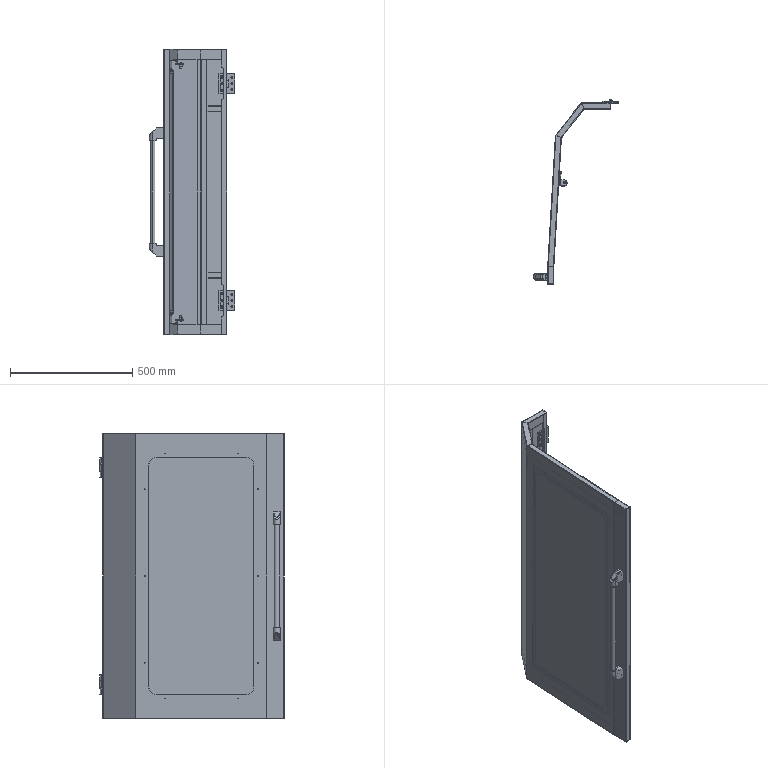Part | SolidWorks | 40 solids | 1078 faces | box 348.6 x 752.5 x 1165 mm | volume 4533101 mm3 | plane 570 | cylinder 412 | cone 84 | spline 12 | commonest cylinder face diameters 4 x50 6 x46 0.4 x37 6.4 x28 4.4 x25 10 x24